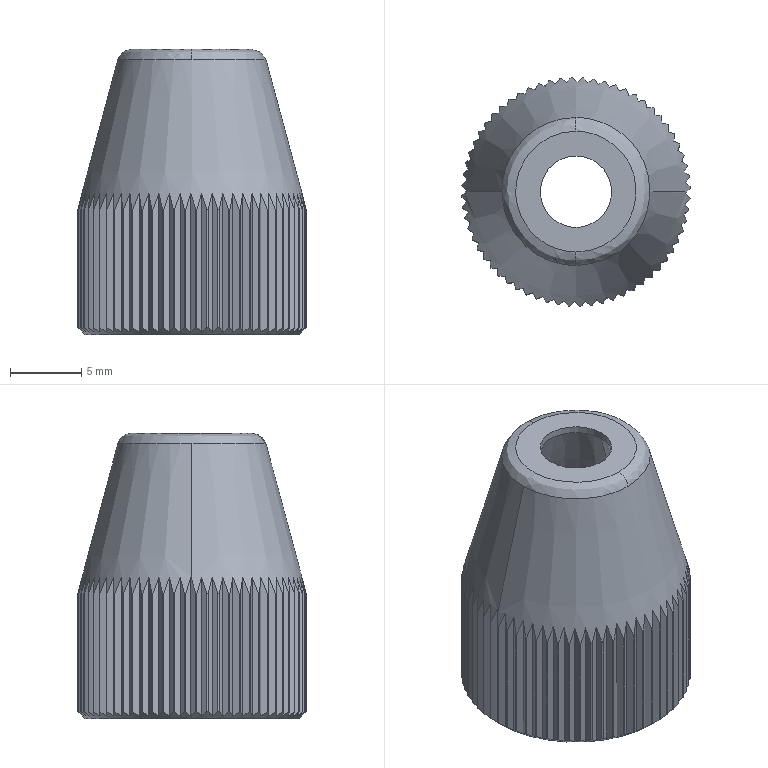Part | SolidWorks | features BaseBody 1 | 1 solid | 212 faces | box 15.991 x 15.991 x 20 mm | volume 2427 mm3 | plane 132 | cylinder 70 | cone 8 | spline 2 | commonest cylinder face diameters 16 x64 5 x2 7.2 x2 8.4 x2